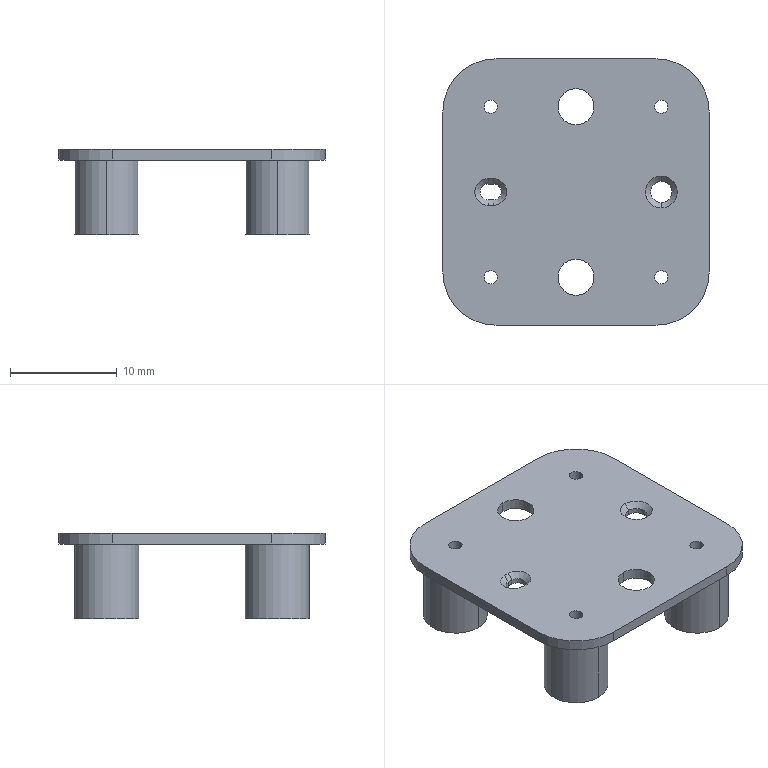NC program | NX | posted with a generic post | part box 25 x 25 x 8 mm
Whole program:
N10 G17 G21 G94 G90
(FLOOR_WALL_COPY , TOOL : D80)
N12 T19 M6
N14 G54
N16 G17 G0 G90 X-59.5 Y0. S6500 M3
N18 G43 Z30. H19
N20 Z3.
N22 G94 G1 Z0. F1500.
N24 X-54.5
N26 X54.5
N28 X59.5
N30 Z3.
N32 G0 Z30.
N34 M5
(DRILLING_COPY_1 , TOOL : D6A45)
N36 T01 M6
N38 G54
N40 G17 G0 G90 X-8. Y-8. S5000 M3
N42 G43 Z30. H1
N44 G94 G81 G98 Z-0.75 F350. R3.
N46 X0.
N48 X8.
N50 Y0.
N52 Y8.
N54 X0.
N56 X-8.
N58 G80
N60 G0 X-8. Y8. Z30.
N62 M5
(DRILLING_COPY_1_COPY_COPY , TOOL : 1.25ZT)
N64 T20 M6
N66 G54
N68 G17 G0 G90 X-8. Y-8. S2000 M3
N70 G43 Z30. H20
N72 G94 G83 G98 Z-9.376 F120. Q2. R3.
N74 Y8.
N76 X8.
N78 Y-8.
N80 G80
N82 G0 X8. Y-8. Z30.
N84 M5
(DRILLING_COPY_1_COPY_1_1_COPY_1 , TOOL : 3.4ZT)
N86 T03 M6
N88 G54
N90 G17 G0 G90 X0. Y-8. S2000 M3
N92 G43 Z30. H3
N94 G94 G83 G98 Z-3.521 F200. Q2. R3.
N96 Y8.
N98 G80
N100 G0 X0. Y8. Z30.
N102 M5
(ZLEVEL_PROFILE_COPY , TOOL : D1.0)
N104 T18 M6
N106 G54
N108 G17 G0 G90 X-7.518 Y-0.136 S9500 M3
N110 G43 Z30. H18
N112 Z0.5
N114 G94 G1 X-7.513 Y-0.131 F1000.
N116 Y0.121 Z0.486
N118 X-7.598 Y0.22 Z0.48
N120 X-7.722 Y0.24 Z0.473
N122 Y0.25
N124 X-8.278 Z0.443
N126 X-8.402 Y0.231 Z0.437
N128 X-8.487 Y0.131 Z0.43
N130 Y-0.12 Z0.417
N132 X-8.402 Y-0.219 Z0.41
N134 X-8.278 Y-0.239 Z0.403
N136 Y-0.25
N138 X-7.722 Z0.374
N140 X-7.598 Y-0.23 Z0.367
N142 X-7.513 Y-0.131 Z0.36
N144 Y0.121 Z0.347
N146 X-7.598 Y0.22 Z0.34
N148 X-7.722 Y0.24 Z0.334
N150 Y0.25 Z0.333
N152 X-8.278 Z0.304
N154 X-8.402 Y0.231 Z0.297
N156 X-8.487 Y0.131 Z0.29
N158 Y-0.12 Z0.277
N160 X-8.402 Y-0.219 Z0.27
N162 X-8.278 Y-0.239 Z0.264
N164 Y-0.25 Z0.263
N166 X-7.722 Z0.234
N168 X-7.598 Y-0.23 Z0.228
N170 X-7.513 Y-0.131 Z0.221
N172 Y0.121 Z0.207
N174 X-7.598 Y0.22 Z0.201
N176 X-7.722 Y0.24 Z0.194
N178 Y0.25
N180 X-8.278 Z0.164
N182 X-8.402 Y0.231 Z0.158
N184 X-8.487 Y0.131 Z0.151
N186 Y-0.12 Z0.138
N188 X-8.402 Y-0.219 Z0.131
N190 X-8.278 Y-0.239 Z0.124
N192 Y-0.25
N194 X-7.722 Z0.095
N196 X-7.598 Y-0.23 Z0.088
N198 X-7.513 Y-0.131 Z0.081
N200 Y0.121 Z0.068
N202 X-7.598 Y0.22 Z0.061
N204 X-7.722 Y0.24 Z0.055
N206 Y0.25 Z0.054
N208 X-8.278 Z0.025
N210 X-8.402 Y0.231 Z0.018
N212 X-8.487 Y0.131 Z0.011
N214 Y-0.12 Z-0.002
N216 X-8.402 Y-0.219 Z-0.009
N218 X-8.278 Y-0.239 Z-0.015
N220 Y-0.25 Z-0.016
N222 X-7.722 Z-0.045
N224 X-7.598 Y-0.23 Z-0.051
N226 X-7.513 Y-0.131 Z-0.058
N228 Y0.121 Z-0.071
N230 X-7.598 Y0.22 Z-0.078
N232 X-7.722 Y0.24 Z-0.085
N234 Y0.25
N236 X-8. Z-0.1
N238 X-8.278
N240 G3 X-8.278 Y-0.239 R0.247
N242 G1 Y-0.25
N244 X-7.722
N246 G3 X-7.722 Y0.24 R0.248
N248 G1 Y0.25
N250 X-8.
N252 X-8.119 Z-0.106
N254 X-8.238 Y0.245 Z-0.113
N256 X-8.385 Y0.195 Z-0.121
N258 X-8.437 Y0.146 Z-0.125
N260 X-8.479 Y0.059 Z-0.13
N262 X-8.489 Y0.015 Z-0.132
N264 X-8.488 Y-0.016 Z-0.134
N266 X-8.475 Y-0.078 Z-0.138
N268 X-8.435 Y-0.148 Z-0.142
N270 X-8.41 Y-0.179 Z-0.144
N272 X-8.378 Y-0.199 Z-0.146
N274 X-8.305 Y-0.231 Z-0.15
N276 X-8.261 Y-0.241 Z-0.153
N278 X-8.08 Y-0.25 Z-0.163
N280 X-7.842 Z-0.175
N282 X-7.663 Y-0.225 Z-0.185
N284 X-7.62 Y-0.198 Z-0.188
N286 X-7.54 Y-0.112 Z-0.194
N288 X-7.513 Y0. Z-0.2
N290 G3 X-7.722 Y0.24 R0.248
N292 G1 Y0.25
N294 X-8.
N296 X-8.119 Z-0.206
N298 X-8.238 Y0.245 Z-0.213
N300 X-8.385 Y0.195 Z-0.221
N302 X-8.437 Y0.146 Z-0.225
N304 X-8.479 Y0.059 Z-0.23
N306 X-8.489 Y0.015 Z-0.232
N308 X-8.488 Y-0.016 Z-0.234
N310 X-8.475 Y-0.078 Z-0.238
N312 X-8.435 Y-0.148 Z-0.242
N314 X-8.41 Y-0.179 Z-0.244
N316 X-8.378 Y-0.199 Z-0.246
N318 X-8.305 Y-0.231 Z-0.25
N320 X-8.261 Y-0.241 Z-0.253
N322 X-8.08 Y-0.25 Z-0.263
N324 X-7.842 Z-0.275
N326 X-7.663 Y-0.225 Z-0.285
N328 X-7.62 Y-0.198 Z-0.288
N330 X-7.54 Y-0.112 Z-0.294
N332 X-7.513 Y0. Z-0.3
N334 G3 X-7.722 Y0.24 R0.248
N336 G1 Y0.25
N338 X-8.
N340 X-8.119 Z-0.306
N342 X-8.238 Y0.245 Z-0.313
N344 X-8.385 Y0.195 Z-0.321
N346 X-8.437 Y0.146 Z-0.325
N348 X-8.479 Y0.059 Z-0.33
N350 X-8.489 Y0.015 Z-0.332
N352 X-8.488 Y-0.016 Z-0.334
N354 X-8.475 Y-0.078 Z-0.338
N356 X-8.435 Y-0.148 Z-0.342
N358 X-8.41 Y-0.179 Z-0.344
N360 X-8.378 Y-0.199 Z-0.346
N362 X-8.305 Y-0.231 Z-0.35
N364 X-8.261 Y-0.24 Z-0.353
N366 X-8.08 Y-0.25 Z-0.363
N368 X-7.842 Z-0.375
N370 X-7.663 Y-0.225 Z-0.385
N372 X-7.62 Y-0.198 Z-0.388
N374 X-7.54 Y-0.112 Z-0.394
N376 X-7.513 Y0. Z-0.4
N378 G3 X-7.722 Y0.24 R0.248
N380 G1 Y0.25
N382 X-8.
N384 X-8.119 Z-0.406
N386 X-8.238 Y0.245 Z-0.413
N388 X-8.385 Y0.195 Z-0.421
N390 X-8.437 Y0.146 Z-0.425
N392 X-8.479 Y0.059 Z-0.43
N394 X-8.488 Y0.016 Z-0.432
N396 X-8.49 Y-0.016 Z-0.434
N398 X-8.475 Y-0.078 Z-0.438
N400 X-8.434 Y-0.151 Z-0.442
N402 X-8.407 Y-0.18 Z-0.444
N404 X-8.376 Y-0.201 Z-0.446
N406 X-8.305 Y-0.231 Z-0.45
N408 X-8.26 Y-0.24 Z-0.453
N410 X-8.08 Y-0.25 Z-0.463
N412 X-7.842 Z-0.475
N414 X-7.666 Y-0.224 Z-0.484
N416 X-7.62 Y-0.198 Z-0.488
N418 X-7.54 Y-0.109 Z-0.494
N420 X-7.5 Y0. Z-0.5
N422 G3 X-7.75 Y0.25 R0.25
N424 G1 X-8.
N426 X-8.12 Z-0.506
N428 X-8.241 Y0.243 Z-0.513
N430 X-8.388 Y0.192 Z-0.521
N432 X-8.44 Y0.142 Z-0.525
N434 X-8.489 Y0.016 Z-0.532
N436 X-8.477 Y-0.075 Z-0.538
N438 X-8.418 Y-0.172 Z-0.544
N440 X-8.317 Y-0.228 Z-0.55
N442 X-8.275 Y-0.236 Z-0.552
N444 X-8.08 Y-0.25 Z-0.563
N446 X-7.839 Z-0.575
N448 X-7.662 Y-0.224 Z-0.584
N450 X-7.615 Y-0.195 Z-0.588
N452 X-7.538 Y-0.108 Z-0.594
N454 X-7.5 Y0. Z-0.6
N456 G3 X-7.75 Y0.25 R0.25
N458 G1 X-8.
N460 X-8.12 Z-0.606
N462 X-8.241 Y0.243 Z-0.613
N464 X-8.388 Y0.192 Z-0.621
N466 X-8.44 Y0.142 Z-0.625
N468 X-8.489 Y0.016 Z-0.632
N470 X-8.477 Y-0.075 Z-0.638
N472 X-8.418 Y-0.172 Z-0.644
N474 X-8.317 Y-0.228 Z-0.65
N476 X-8.275 Y-0.238 Z-0.652
N478 X-8.08 Y-0.25 Z-0.663
N480 X-7.839 Z-0.675
N482 X-7.662 Y-0.224 Z-0.684
N484 X-7.615 Y-0.195 Z-0.688
N486 X-7.538 Y-0.108 Z-0.694
N488 X-7.5 Y0. Z-0.7
N490 G3 X-7.75 Y0.25 R0.25
N492 G1 X-8.
N494 X-8.12 Z-0.706
N496 X-8.241 Y0.243 Z-0.713
N498 X-8.388 Y0.192 Z-0.721
N500 X-8.44 Y0.142 Z-0.725
N502 X-8.489 Y0.016 Z-0.732
N504 X-8.477 Y-0.075 Z-0.738
N506 X-8.418 Y-0.172 Z-0.744
N508 X-8.317 Y-0.228 Z-0.75
N510 X-8.274 Y-0.238 Z-0.752
N512 X-8.08 Y-0.25 Z-0.763
N514 X-7.839 Z-0.775
N516 X-7.662 Y-0.224 Z-0.784
N518 X-7.615 Y-0.195 Z-0.788
N520 X-7.538 Y-0.108 Z-0.794
N522 X-7.5 Y0. Z-0.8
N524 G3 X-7.75 Y0.25 R0.25
N526 G1 X-8.
N528 X-8.12 Z-0.806
N530 X-8.241 Y0.243 Z-0.813
N532 X-8.389 Y0.193 Z-0.821
N534 X-8.44 Y0.142 Z-0.825
N536 X-8.489 Y0.013 Z-0.832
N538 X-8.477 Y-0.075 Z-0.838
N540 X-8.417 Y-0.172 Z-0.844
N542 X-8.317 Y-0.228 Z-0.85
N544 X-8.274 Y-0.238 Z-0.852
N546 X-8.08 Y-0.25 Z-0.863
N548 X-7.839 Z-0.875
N550 X-7.662 Y-0.224 Z-0.884
N552 X-7.615 Y-0.195 Z-0.888
N554 X-7.538 Y-0.108 Z-0.894
N556 X-7.5 Y0. Z-0.9
N558 G3 X-7.75 Y0.25 R0.25
N560 G1 X-8.
N562 X-8.12 Z-0.906
N564 X-8.241 Y0.243 Z-0.913
N566 X-8.389 Y0.193 Z-0.921
N568 X-8.44 Y0.142 Z-0.925
N570 X-8.489 Y0.013 Z-0.932
N572 X-8.477 Y-0.075 Z-0.938
N574 X-8.44 Y-0.143 Z-0.942
N576 X-8.419 Y-0.173 Z-0.944
N578 X-8.387 Y-0.193 Z-0.946
N580 X-8.317 Y-0.228 Z-0.95
N582 X-8.269 Y-0.238 Z-0.953
N584 X-8.08 Y-0.25 Z-0.963
N586 X-7.839 Z-0.975
N588 X-7.662 Y-0.224 Z-0.984
N590 X-7.615 Y-0.195 Z-0.988
N592 X-7.538 Y-0.108 Z-0.994
N594 X-7.5 Y0. Z-1.
N596 G3 X-7.75 Y0.25 R0.25
N598 G1 X-8.25
N600 G3 X-8.5 Y0. R0.25
N602 X-8.25 Y-0.25 R0.25
N604 G1 X-7.75
N606 G3 X-7.5 Y0. R0.25
N608 G1 Z-0.5
N610 G0 Z30.
N612 X7.651 Y0.313
N614 Z0.5
N616 G1 X7.51 Y0.157 Z0.489
N618 X7.521 Y-0.192 Z0.471
N620 X7.825 Y-0.492 Z0.448
N622 X8. Y-0.495 Z0.439
N624 X8.174 Y-0.492 Z0.43
N626 X8.485 Y-0.177 Z0.407
N628 Y0.012 Z0.397
N630 X8.479 Y0.187 Z0.388
N632 X8.144 Y0.497 Z0.364
N634 X7.97 Y0.489 Z0.355
N636 X7.796 Y0.475 Z0.346
N638 X7.51 Y0.157 Z0.323
N640 X7.521 Y-0.192 Z0.305
N642 X7.825 Y-0.492 Z0.282
N644 X8. Y-0.495 Z0.273
N646 X8.174 Y-0.492 Z0.264
N648 X8.485 Y-0.177 Z0.241
N650 Y0.012 Z0.231
N652 X8.479 Y0.187 Z0.222
N654 X8.144 Y0.497 Z0.198
N656 X7.97 Y0.489 Z0.189
N658 X7.796 Y0.475 Z0.18
N660 X7.51 Y0.157 Z0.157
N662 X7.521 Y-0.192 Z0.139
N664 X7.825 Y-0.492 Z0.117
N666 X8. Y-0.495 Z0.107
N668 X8.174 Y-0.492 Z0.098
N670 X8.485 Y-0.177 Z0.075
N672 Y0.012 Z0.065
N674 X8.479 Y0.187 Z0.056
N676 X8.144 Y0.497 Z0.032
N678 X7.97 Y0.489 Z0.023
N680 X7.796 Y0.475 Z0.014
N682 X7.51 Y0.157 Z-0.009
N684 X7.521 Y-0.192 Z-0.027
N686 X7.825 Y-0.492 Z-0.049
N688 X8. Y-0.495 Z-0.059
N690 X8.174 Y-0.492 Z-0.068
N692 X8.485 Y-0.177 Z-0.091
N694 Y-0.003 Z-0.1
N696 Y0.012
N698 G3 X7.97 Y0.489 R0.492
N700 X8. Y-0.495 R0.493
N702 X8.485 Y-0.003 R0.492
N704 G1 X8.461 Y0.154 Z-0.107
N706 X8.434 Y0.22 Z-0.11
N708 X8.36 Y0.328 Z-0.116
N710 X8.284 Y0.39 Z-0.12
N712 X8.162 Y0.461 Z-0.126
N714 X8.075 Y0.477 Z-0.13
N716 X7.931 Y0.479 Z-0.136
N718 X7.851 Y0.461 Z-0.14
N720 X7.722 Y0.395 Z-0.146
N722 X7.652 Y0.348 Z-0.15
N724 X7.588 Y0.252 Z-0.155
N726 X7.538 Y0.148 Z-0.16
N728 X7.513 Y0.027 Z-0.165
N730 X7.525 Y-0.078 Z-0.17
N732 X7.562 Y-0.213 Z-0.176
N734 X7.612 Y-0.286 Z-0.18
N736 X7.709 Y-0.385 Z-0.186
N738 X7.783 Y-0.433 Z-0.19
N740 X7.89 Y-0.471 Z-0.195
N742 X8. Y-0.495 Z-0.2
N744 G3 X8.485 Y-0.003 R0.492
N746 G1 X8.461 Y0.154 Z-0.207
N748 X8.434 Y0.22 Z-0.21
N750 X8.36 Y0.327 Z-0.216
N752 X8.284 Y0.39 Z-0.22
N754 X8.162 Y0.461 Z-0.226
N756 X8.075 Y0.477 Z-0.23
N758 X7.931 Y0.479 Z-0.236
N760 X7.851 Y0.461 Z-0.24
N762 X7.723 Y0.395 Z-0.246
N764 X7.652 Y0.348 Z-0.25
N766 X7.588 Y0.252 Z-0.255
N768 X7.538 Y0.148 Z-0.26
N770 X7.513 Y0.027 Z-0.265
N772 X7.525 Y-0.078 Z-0.27
N774 X7.562 Y-0.213 Z-0.276
N776 X7.612 Y-0.286 Z-0.28
N778 X7.709 Y-0.385 Z-0.286
N780 X7.783 Y-0.433 Z-0.29
N782 X7.89 Y-0.47 Z-0.295
N784 X8. Y-0.495 Z-0.3
N786 G3 X8.485 Y-0.003 R0.492
N788 G1 X8.461 Y0.154 Z-0.307
N790 X8.434 Y0.22 Z-0.31
N792 X8.36 Y0.327 Z-0.316
N794 X8.284 Y0.39 Z-0.32
N796 X8.162 Y0.461 Z-0.326
N798 X8.075 Y0.477 Z-0.33
N800 X7.932 Y0.479 Z-0.336
N802 X7.851 Y0.461 Z-0.34
N804 X7.723 Y0.395 Z-0.346
N806 X7.652 Y0.348 Z-0.35
N808 X7.588 Y0.252 Z-0.355
N810 X7.538 Y0.148 Z-0.36
N812 X7.513 Y0.027 Z-0.365
N814 X7.525 Y-0.078 Z-0.37
N816 X7.562 Y-0.213 Z-0.376
N818 X7.612 Y-0.286 Z-0.38
N820 X7.709 Y-0.385 Z-0.386
N822 X7.783 Y-0.433 Z-0.39
N824 X7.89 Y-0.47 Z-0.395
N826 X8. Y-0.495 Z-0.4
N828 G3 X8.485 Y-0.003 R0.492
N830 G1 X8.461 Y0.151 Z-0.407
N832 X8.433 Y0.219 Z-0.41
N834 X8.358 Y0.328 Z-0.416
N836 X8.284 Y0.39 Z-0.42
N838 X8.162 Y0.461 Z-0.426
N840 X8.075 Y0.478 Z-0.43
N842 X7.932 Y0.477 Z-0.436
N844 X7.85 Y0.462 Z-0.44
N846 X7.727 Y0.398 Z-0.446
N848 X7.652 Y0.347 Z-0.45
N850 X7.588 Y0.251 Z-0.455
N852 X7.538 Y0.149 Z-0.46
N854 X7.515 Y0.028 Z-0.465
N856 X7.524 Y-0.078 Z-0.47
N858 X7.561 Y-0.211 Z-0.476
N860 X7.611 Y-0.287 Z-0.48
N862 X7.706 Y-0.383 Z-0.486
N864 X7.782 Y-0.433 Z-0.49
N866 X7.89 Y-0.47 Z-0.495
N868 X8. Y-0.5 Z-0.5
N870 X8.015
N872 G3 X8.5 Y-0.003 R0.5
N874 G1 X8.466 Y0.127 Z-0.506
N876 X8.434 Y0.218 Z-0.51
N878 X8.364 Y0.323 Z-0.516
N880 X8.286 Y0.389 Z-0.52
N882 X8.169 Y0.459 Z-0.526
N884 X8.078 Y0.477 Z-0.53
N886 X7.935 Y0.479 Z-0.536
N888 X7.853 Y0.462 Z-0.54
N890 X7.733 Y0.401 Z-0.546
N892 X7.655 Y0.349 Z-0.55
N894 X7.525 Y0.157 Z-0.56
N896 X7.504 Y0.063 Z-0.564
N898 X7.522 Y-0.073 Z-0.57
N900 X7.561 Y-0.211 Z-0.576
N902 X7.609 Y-0.281 Z-0.58
N904 X7.708 Y-0.385 Z-0.586
N906 X7.777 Y-0.431 Z-0.59
N908 X7.886 Y-0.469 Z-0.595
N910 X7.997 Y-0.5 Z-0.6
N912 X8.015
N914 G3 X8.5 Y-0.003 R0.5
N916 G1 X8.466 Y0.127 Z-0.606
N918 X8.434 Y0.218 Z-0.61
N920 X8.364 Y0.323 Z-0.616
N922 X8.286 Y0.389 Z-0.62
N924 X8.169 Y0.459 Z-0.626
N926 X8.078 Y0.477 Z-0.63
N928 X7.935 Y0.479 Z-0.636
N930 X7.853 Y0.462 Z-0.64
N932 X7.733 Y0.401 Z-0.646
N934 X7.655 Y0.349 Z-0.65
N936 X7.525 Y0.157 Z-0.66
N938 X7.504 Y0.063 Z-0.664
N940 X7.522 Y-0.073 Z-0.67
N942 X7.561 Y-0.211 Z-0.676
N944 X7.609 Y-0.281 Z-0.68
N946 X7.708 Y-0.385 Z-0.686
N948 X7.777 Y-0.431 Z-0.69
N950 X7.886 Y-0.469 Z-0.695
N952 X7.997 Y-0.5 Z-0.7
N954 X8.015
N956 G3 X8.5 Y-0.003 R0.5
N958 G1 X8.466 Y0.126 Z-0.706
N960 X8.434 Y0.218 Z-0.71
N962 X8.364 Y0.323 Z-0.716
N964 X8.286 Y0.389 Z-0.72
N966 X8.168 Y0.458 Z-0.726
N968 X8.078 Y0.477 Z-0.73
N970 X7.936 Y0.479 Z-0.736
N972 X7.853 Y0.462 Z-0.74
N974 X7.733 Y0.401 Z-0.746
N976 X7.655 Y0.349 Z-0.75
N978 X7.525 Y0.157 Z-0.76
N980 X7.504 Y0.063 Z-0.764
N982 X7.522 Y-0.073 Z-0.77
N984 X7.561 Y-0.211 Z-0.776
N986 X7.609 Y-0.281 Z-0.78
N988 X7.708 Y-0.385 Z-0.786
N990 X7.777 Y-0.431 Z-0.79
N992 X7.886 Y-0.468 Z-0.795
N994 X7.997 Y-0.5 Z-0.8
N996 X8.015
N998 G3 X8.5 Y-0.003 R0.5
N1000 G1 X8.466 Y0.126 Z-0.806
N1002 X8.434 Y0.218 Z-0.81
N1004 X8.364 Y0.323 Z-0.816
N1006 X8.286 Y0.389 Z-0.82
N1008 X8.168 Y0.458 Z-0.826
N1010 X8.078 Y0.477 Z-0.83
N1012 X7.936 Y0.479 Z-0.836
N1014 X7.853 Y0.462 Z-0.84
N1016 X7.733 Y0.401 Z-0.846
N1018 X7.655 Y0.349 Z-0.85
N1020 X7.525 Y0.157 Z-0.86
N1022 X7.504 Y0.063 Z-0.864
N1024 X7.522 Y-0.073 Z-0.87
N1026 X7.561 Y-0.211 Z-0.876
N1028 X7.609 Y-0.281 Z-0.88
N1030 X7.708 Y-0.385 Z-0.886
N1032 X7.777 Y-0.431 Z-0.89
N1034 X7.886 Y-0.468 Z-0.895
N1036 X7.997 Y-0.5 Z-0.9
N1038 X8.015
N1040 G3 X8.5 Y-0.003 R0.5
N1042 G1 X8.466 Y0.126 Z-0.906
N1044 X8.434 Y0.218 Z-0.91
N1046 X8.364 Y0.323 Z-0.916
N1048 X8.286 Y0.389 Z-0.92
N1050 X8.168 Y0.458 Z-0.926
N1052 X8.078 Y0.477 Z-0.93
N1054 X7.936 Y0.479 Z-0.936
N1056 X7.853 Y0.462 Z-0.94
N1058 X7.733 Y0.401 Z-0.946
N1060 X7.655 Y0.349 Z-0.95
N1062 X7.525 Y0.157 Z-0.96
N1064 X7.504 Y0.063 Z-0.964
N1066 X7.522 Y-0.073 Z-0.97
N1068 X7.561 Y-0.211 Z-0.976
N1070 X7.609 Y-0.281 Z-0.98
N1072 X7.708 Y-0.385 Z-0.986
N1074 X7.777 Y-0.431 Z-0.99
N1076 X7.886 Y-0.468 Z-0.995
N1078 X7.997 Y-0.5 Z-1.
N1080 X8.015
N1082 G3 X7.997 Y-0.5 R-0.5
N1084 G1 Z-0.5
N1086 G0 Z30.
N1088 M5
(ZLEVEL_PROFILE , TOOL : D10)
N1090 T15 M6
N1092 G54
N1094 G17 G0 G90 X15.543 Y-13.61 S9500 M3
N1096 G43 Z30. H15
N1098 Z1.5
N1100 G94 G1 X15.35 Y-13.903 Z1.482 F1000.
N1102 X13.903 Y-15.35 Z1.374
N1104 X12.194 Y-16.477 Z1.267
N1106 X10.293 Y-17.237 Z1.16
N1108 X8.279 Y-17.6 Z1.053
N1110 X-8.279 Z0.185
N1112 X-10.293 Y-17.237 Z0.078
N1114 X-12.194 Y-16.477 Z-0.03
N1116 X-13.903 Y-15.35 Z-0.137
N1118 X-15.35 Y-13.903 Z-0.244
N1120 X-16.477 Y-12.194 Z-0.352
N1122 X-17.237 Y-10.293 Z-0.459
N1124 X-17.6 Y-8.279 Z-0.566
N1126 Y0. Z-1.
N1128 Y7.5 F3200.
N1130 G2 X-7.5 Y17.6 R10.1
N1132 G1 X7.5
N1134 G2 X17.6 Y7.5 R10.1
N1136 G1 Y-7.5
N1138 G2 X7.5 Y-17.6 R10.1
N1140 G1 X-7.5
N1142 G2 X-17.6 Y-7.5 R10.1
N1144 G1 Y0.
N1146 Y6.968 Z-1.122
N1148 Y7.355 Z-1.128
N1150 X-17.597 Y7.742 Z-1.135
N1152 X-17.58 Y8.129 Z-1.142
N1154 X-17.549 Y8.514 Z-1.149
N1156 X-17.503 Y8.899 Z-1.155
N1158 X-17.442 Y9.281 Z-1.162
N1160 X-17.366 Y9.661 Z-1.169
N1162 X-17.276 Y10.037 Z-1.176
N1164 X-17.172 Y10.41 Z-1.182
N1166 X-17.053 Y10.778 Z-1.189
N1168 X-16.921 Y11.142 Z-1.196
N1170 X-16.774 Y11.5 Z-1.203
N1172 X-16.614 Y11.853 Z-1.209
N1174 X-16.441 Y12.199 Z-1.216
N1176 X-16.254 Y12.538 Z-1.223
N1178 X-16.055 Y12.869 Z-1.23
N1180 X-15.842 Y13.193 Z-1.236
N1182 X-15.618 Y13.509 Z-1.243
N1184 X-15.382 Y13.815 Z-1.25
N1186 X-15.134 Y14.113 Z-1.257
N1188 X-14.875 Y14.4 Z-1.264
N1190 X-14.605 Y14.678 Z-1.27
N1192 X-14.325 Y14.945 Z-1.277
N1194 X-14.035 Y15.201 Z-1.284
N1196 X-13.735 Y15.446 Z-1.291
N1198 X-13.426 Y15.679 Z-1.297
N1200 X-13.108 Y15.9 Z-1.304
N1202 X-12.782 Y16.109 Z-1.311
N1204 X-12.449 Y16.305 Z-1.318
N1206 X-12.108 Y16.488 Z-1.324
N1208 X-11.76 Y16.658 Z-1.331
N1210 X-11.406 Y16.814 Z-1.338
N1212 X-11.046 Y16.957 Z-1.345
N1214 X-10.681 Y17.086 Z-1.351
N1216 X-10.311 Y17.201 Z-1.358
N1218 X-9.938 Y17.301 Z-1.365
N1220 X-9.56 Y17.388 Z-1.372
N1222 X-9.18 Y17.459 Z-1.378
N1224 X-8.797 Y17.516 Z-1.385
N1226 X-8.412 Y17.559 Z-1.392
N1228 X-8.026 Y17.586 Z-1.399
N1230 X-7.639 Y17.599 Z-1.405
N1232 X-7.252 Y17.6 Z-1.412
N1234 X-6.478 Z-1.426
N1236 X7.07 Z-1.662
N1238 X7.457 Z-1.669
N1240 X7.844 Y17.594 Z-1.676
N1242 X8.231 Y17.574 Z-1.682
N1244 X8.616 Y17.538 Z-1.689
N1246 X9. Y17.488 Z-1.696
N1248 X9.382 Y17.423 Z-1.703
N1250 X9.761 Y17.344 Z-1.709
N1252 X10.136 Y17.25 Z-1.716
N1254 X10.508 Y17.142 Z-1.723
N1256 X10.875 Y17.019 Z-1.73
N1258 X11.237 Y16.883 Z-1.736
N1260 X11.594 Y16.733 Z-1.743
N1262 X11.945 Y16.569 Z-1.75
N1264 X12.289 Y16.392 Z-1.757
N1266 X12.626 Y16.202 Z-1.764
N1268 X12.956 Y16. Z-1.77
N1270 X13.278 Y15.784 Z-1.777
N1272 X13.591 Y15.557 Z-1.784
N1274 X13.895 Y15.318 Z-1.791
N1276 X14.19 Y15.067 Z-1.797
N1278 X14.475 Y14.805 Z-1.804
N1280 X14.75 Y14.532 Z-1.811
N1282 X15.014 Y14.249 Z-1.818
N1284 X15.267 Y13.956 Z-1.824
N1286 X15.509 Y13.654 Z-1.831
N1288 X15.739 Y13.343 Z-1.838
N1290 X15.956 Y13.023 Z-1.845
N1292 X16.162 Y12.695 Z-1.851
N1294 X16.354 Y12.359 Z-1.858
N1296 X16.534 Y12.016 Z-1.865
N1298 X16.7 Y11.667 Z-1.872
N1300 X16.853 Y11.311 Z-1.878
N1302 X16.993 Y10.95 Z-1.885
N1304 X17.118 Y10.584 Z-1.892
N1306 X17.229 Y10.213 Z-1.899
N1308 X17.326 Y9.838 Z-1.905
N1310 X17.408 Y9.46 Z-1.912
N1312 X17.476 Y9.079 Z-1.919
N1314 X17.529 Y8.695 Z-1.926
N1316 X17.567 Y8.31 Z-1.932
N1318 X17.591 Y7.924 Z-1.939
N1320 X17.6 Y7.537 Z-1.946
N1322 Y7.15 Z-1.953
N1324 Y4.44 Z-2.
N1326 Y-7.5
N1328 G2 X7.5 Y-17.6 R10.1
N1330 G1 X-7.5
N1332 G2 X-17.6 Y-7.5 R10.1
N1334 G1 Y0.
N1336 Y6.968 Z-2.122
N1338 Y7.355 Z-2.128
N1340 X-17.597 Y7.742 Z-2.135
N1342 X-17.58 Y8.129 Z-2.142
N1344 X-17.549 Y8.514 Z-2.149
N1346 X-17.503 Y8.899 Z-2.155
N1348 X-17.442 Y9.281 Z-2.162
N1350 X-17.366 Y9.661 Z-2.169
N1352 X-17.276 Y10.037 Z-2.176
N1354 X-17.172 Y10.41 Z-2.182
N1356 X-17.053 Y10.778 Z-2.189
N1358 X-16.921 Y11.142 Z-2.196
N1360 X-16.774 Y11.5 Z-2.203
N1362 X-16.614 Y11.853 Z-2.209
N1364 X-16.441 Y12.199 Z-2.216
N1366 X-16.254 Y12.538 Z-2.223
N1368 X-16.055 Y12.869 Z-2.23
N1370 X-15.842 Y13.193 Z-2.236
N1372 X-15.618 Y13.509 Z-2.243
N1374 X-15.382 Y13.815 Z-2.25
N1376 X-15.134 Y14.113 Z-2.257
N1378 X-14.875 Y14.4 Z-2.264
N1380 X-14.605 Y14.678 Z-2.27
N1382 X-14.325 Y14.945 Z-2.277
N1384 X-14.035 Y15.201 Z-2.284
N1386 X-13.735 Y15.446 Z-2.291
N1388 X-13.426 Y15.679 Z-2.297
N1390 X-13.108 Y15.9 Z-2.304
N1392 X-12.782 Y16.109 Z-2.311
N1394 X-12.449 Y16.305 Z-2.318
N1396 X-12.108 Y16.488 Z-2.324
N1398 X-11.76 Y16.658 Z-2.331
N1400 X-11.406 Y16.814 Z-2.338
N1402 X-11.046 Y16.957 Z-2.345
N1404 X-10.681 Y17.086 Z-2.351
N1406 X-10.311 Y17.201 Z-2.358
N1408 X-9.938 Y17.301 Z-2.365
N1410 X-9.56 Y17.388 Z-2.372
N1412 X-9.18 Y17.459 Z-2.378
N1414 X-8.797 Y17.516 Z-2.385
N1416 X-8.412 Y17.559 Z-2.392
N1418 X-8.026 Y17.586 Z-2.399
N1420 X-7.639 Y17.599 Z-2.405
N1422 X-7.252 Y17.6 Z-2.412
N1424 X-6.478 Z-2.426
N1426 X7.07 Z-2.662
N1428 X7.457 Z-2.669
N1430 X7.844 Y17.594 Z-2.676
N1432 X8.231 Y17.574 Z-2.682
N1434 X8.616 Y17.538 Z-2.689
N1436 X9. Y17.488 Z-2.696
N1438 X9.382 Y17.423 Z-2.703
N1440 X9.761 Y17.344 Z-2.709
N1442 X10.136 Y17.25 Z-2.716
N1444 X10.508 Y17.142 Z-2.723
N1446 X10.875 Y17.019 Z-2.73
N1448 X11.237 Y16.883 Z-2.736
N1450 X11.594 Y16.733 Z-2.743
N1452 X11.945 Y16.569 Z-2.75
N1454 X12.289 Y16.392 Z-2.757
N1456 X12.626 Y16.202 Z-2.764
N1458 X12.956 Y16. Z-2.77
N1460 X13.278 Y15.784 Z-2.777
N1462 X13.591 Y15.557 Z-2.784
N1464 X13.895 Y15.318 Z-2.791
N1466 X14.19 Y15.067 Z-2.797
N1468 X14.475 Y14.805 Z-2.804
N1470 X14.75 Y14.532 Z-2.811
N1472 X15.014 Y14.249 Z-2.818
N1474 X15.267 Y13.956 Z-2.824
N1476 X15.509 Y13.654 Z-2.831
N1478 X15.739 Y13.343 Z-2.838
N1480 X15.956 Y13.023 Z-2.845
N1482 X16.162 Y12.695 Z-2.851
N1484 X16.354 Y12.359 Z-2.858
N1486 X16.534 Y12.016 Z-2.865
N1488 X16.7 Y11.667 Z-2.872
N1490 X16.853 Y11.311 Z-2.878
N1492 X16.993 Y10.95 Z-2.885
N1494 X17.118 Y10.584 Z-2.892
N1496 X17.229 Y10.213 Z-2.899
N1498 X17.326 Y9.838 Z-2.905
N1500 X17.408 Y9.46 Z-2.912
N1502 X17.476 Y9.079 Z-2.919
N1504 X17.529 Y8.695 Z-2.926
N1506 X17.567 Y8.31 Z-2.932
N1508 X17.591 Y7.924 Z-2.939
N1510 X17.6 Y7.537 Z-2.946
N1512 Y7.15 Z-2.953
N1514 Y4.44 Z-3.
N1516 Y-7.5
N1518 G2 X7.5 Y-17.6 R10.1
N1520 G1 X-7.5
N1522 G2 X-17.6 Y-7.5 R10.1
N1524 G1 Y0.
N1526 Y6.968 Z-3.122
N1528 Y7.355 Z-3.128
N1530 X-17.597 Y7.742 Z-3.135
N1532 X-17.58 Y8.129 Z-3.142
N1534 X-17.549 Y8.514 Z-3.149
N1536 X-17.503 Y8.899 Z-3.155
N1538 X-17.442 Y9.281 Z-3.162
N1540 X-17.366 Y9.661 Z-3.169
N1542 X-17.276 Y10.037 Z-3.176
N1544 X-17.172 Y10.41 Z-3.182
N1546 X-17.053 Y10.778 Z-3.189
N1548 X-16.921 Y11.142 Z-3.196
N1550 X-16.774 Y11.5 Z-3.203
N1552 X-16.614 Y11.853 Z-3.209
N1554 X-16.441 Y12.199 Z-3.216
N1556 X-16.254 Y12.538 Z-3.223
N1558 X-16.055 Y12.869 Z-3.23
N1560 X-15.842 Y13.193 Z-3.236
N1562 X-15.618 Y13.509 Z-3.243
N1564 X-15.382 Y13.815 Z-3.25
N1566 X-15.134 Y14.113 Z-3.257
N1568 X-14.875 Y14.4 Z-3.264
N1570 X-14.605 Y14.678 Z-3.27
N1572 X-14.325 Y14.945 Z-3.277
N1574 X-14.035 Y15.201 Z-3.284
N1576 X-13.735 Y15.446 Z-3.291
N1578 X-13.426 Y15.679 Z-3.297
N1580 X-13.108 Y15.9 Z-3.304
N1582 X-12.782 Y16.109 Z-3.311
N1584 X-12.449 Y16.305 Z-3.318
N1586 X-12.108 Y16.488 Z-3.324
N1588 X-11.76 Y16.658 Z-3.331
N1590 X-11.406 Y16.814 Z-3.338
N1592 X-11.046 Y16.957 Z-3.345
N1594 X-10.681 Y17.086 Z-3.351
N1596 X-10.311 Y17.201 Z-3.358
N1598 X-9.938 Y17.301 Z-3.365
N1600 X-9.56 Y17.388 Z-3.372
N1602 X-9.18 Y17.459 Z-3.378
N1604 X-8.797 Y17.516 Z-3.385
N1606 X-8.412 Y17.559 Z-3.392
N1608 X-8.026 Y17.586 Z-3.399
N1610 X-7.639 Y17.599 Z-3.405
N1612 X-7.252 Y17.6 Z-3.412
N1614 X-6.478 Z-3.426
N1616 X7.07 Z-3.662
N1618 X7.457 Z-3.669
N1620 X7.844 Y17.594 Z-3.676
N1622 X8.231 Y17.574 Z-3.682
N1624 X8.616 Y17.538 Z-3.689
N1626 X9. Y17.488 Z-3.696
N1628 X9.382 Y17.423 Z-3.703
N1630 X9.761 Y17.344 Z-3.709
N1632 X10.136 Y17.25 Z-3.716
N1634 X10.508 Y17.142 Z-3.723
N1636 X10.875 Y17.019 Z-3.73
N1638 X11.237 Y16.883 Z-3.736
N1640 X11.594 Y16.733 Z-3.743
N1642 X11.945 Y16.569 Z-3.75
N1644 X12.289 Y16.392 Z-3.757
N1646 X12.626 Y16.202 Z-3.764
N1648 X12.956 Y16. Z-3.77
N1650 X13.278 Y15.784 Z-3.777
N1652 X13.591 Y15.557 Z-3.784
N1654 X13.895 Y15.318 Z-3.791
N1656 X14.19 Y15.067 Z-3.797
N1658 X14.475 Y14.805 Z-3.804
N1660 X14.75 Y14.532 Z-3.811
N1662 X15.014 Y14.249 Z-3.818
N1664 X15.267 Y13.956 Z-3.824
N1666 X15.509 Y13.654 Z-3.831
N1668 X15.739 Y13.343 Z-3.838
N1670 X15.956 Y13.023 Z-3.845
N1672 X16.162 Y12.695 Z-3.851
N1674 X16.354 Y12.359 Z-3.858
N1676 X16.534 Y12.016 Z-3.865
N1678 X16.7 Y11.667 Z-3.872
N1680 X16.853 Y11.311 Z-3.878
N1682 X16.993 Y10.95 Z-3.885
N1684 X17.118 Y10.584 Z-3.892
N1686 X17.229 Y10.213 Z-3.899
N1688 X17.326 Y9.838 Z-3.905
N1690 X17.408 Y9.46 Z-3.912
N1692 X17.476 Y9.079 Z-3.919
N1694 X17.529 Y8.695 Z-3.926
N1696 X17.567 Y8.31 Z-3.932
N1698 X17.591 Y7.924 Z-3.939
N1700 X17.6 Y7.537 Z-3.946
N1702 Y7.15 Z-3.953
N1704 Y4.44 Z-4.
N1706 Y-7.5
N1708 G2 X7.5 Y-17.6 R10.1
N1710 G1 X-7.5
N1712 G2 X-17.6 Y-7.5 R10.1
N1714 G1 Y0.
N1716 Y6.968 Z-4.122
N1718 Y7.355 Z-4.128
N1720 X-17.597 Y7.742 Z-4.135
N1722 X-17.58 Y8.129 Z-4.142
N1724 X-17.549 Y8.514 Z-4.149
N1726 X-17.503 Y8.899 Z-4.155
N1728 X-17.442 Y9.281 Z-4.162
N1730 X-17.366 Y9.661 Z-4.169
N1732 X-17.276 Y10.037 Z-4.176
N1734 X-17.172 Y10.41 Z-4.182
N1736 X-17.053 Y10.778 Z-4.189
N1738 X-16.921 Y11.142 Z-4.196
N1740 X-16.774 Y11.5 Z-4.203
N1742 X-16.614 Y11.853 Z-4.209
N1744 X-16.441 Y12.199 Z-4.216
N1746 X-16.254 Y12.538 Z-4.223
N1748 X-16.055 Y12.869 Z-4.23
N1750 X-15.842 Y13.193 Z-4.236
N1752 X-15.618 Y13.509 Z-4.243
N1754 X-15.382 Y13.815 Z-4.25
N1756 X-15.134 Y14.113 Z-4.257
N1758 X-14.875 Y14.4 Z-4.264
N1760 X-14.605 Y14.678 Z-4.27
N1762 X-14.325 Y14.945 Z-4.277
N1764 X-14.035 Y15.201 Z-4.284
N1766 X-13.735 Y15.446 Z-4.291
N1768 X-13.426 Y15.679 Z-4.297
N1770 X-13.108 Y15.9 Z-4.304
N1772 X-12.782 Y16.109 Z-4.311
N1774 X-12.449 Y16.305 Z-4.318
N1776 X-12.108 Y16.488 Z-4.324
N1778 X-11.76 Y16.658 Z-4.331
N1780 X-11.406 Y16.814 Z-4.338
N1782 X-11.046 Y16.957 Z-4.345
N1784 X-10.681 Y17.086 Z-4.351
N1786 X-10.311 Y17.201 Z-4.358
N1788 X-9.938 Y17.301 Z-4.365
N1790 X-9.56 Y17.388 Z-4.372
N1792 X-9.18 Y17.459 Z-4.378
N1794 X-8.797 Y17.516 Z-4.385
N1796 X-8.412 Y17.559 Z-4.392
N1798 X-8.026 Y17.586 Z-4.399
N1800 X-7.639 Y17.599 Z-4.405
N1802 X-7.252 Y17.6 Z-4.412
N1804 X-6.478 Z-4.426
N1806 X7.07 Z-4.662
N1808 X7.457 Z-4.669
N1810 X7.844 Y17.594 Z-4.676
N1812 X8.231 Y17.574 Z-4.682
N1814 X8.616 Y17.538 Z-4.689
N1816 X9. Y17.488 Z-4.696
N1818 X9.382 Y17.423 Z-4.703
N1820 X9.761 Y17.344 Z-4.709
N1822 X10.136 Y17.25 Z-4.716
N1824 X10.508 Y17.142 Z-4.723
N1826 X10.875 Y17.019 Z-4.73
N1828 X11.237 Y16.883 Z-4.736
N1830 X11.594 Y16.733 Z-4.743
N1832 X11.945 Y16.569 Z-4.75
N1834 X12.289 Y16.392 Z-4.757
N1836 X12.626 Y16.202 Z-4.764
N1838 X12.956 Y16. Z-4.77
N1840 X13.278 Y15.784 Z-4.777
N1842 X13.591 Y15.557 Z-4.784
N1844 X13.895 Y15.318 Z-4.791
N1846 X14.19 Y15.067 Z-4.797
N1848 X14.475 Y14.805 Z-4.804
N1850 X14.75 Y14.532 Z-4.811
N1852 X15.014 Y14.249 Z-4.818
N1854 X15.267 Y13.956 Z-4.824
N1856 X15.509 Y13.654 Z-4.831
N1858 X15.739 Y13.343 Z-4.838
N1860 X15.956 Y13.023 Z-4.845
N1862 X16.162 Y12.695 Z-4.851
N1864 X16.354 Y12.359 Z-4.858
N1866 X16.534 Y12.016 Z-4.865
N1868 X16.7 Y11.667 Z-4.872
N1870 X16.853 Y11.311 Z-4.878
N1872 X16.993 Y10.95 Z-4.885
N1874 X17.118 Y10.584 Z-4.892
N1876 X17.229 Y10.213 Z-4.899
N1878 X17.326 Y9.838 Z-4.905
N1880 X17.408 Y9.46 Z-4.912
N1882 X17.476 Y9.079 Z-4.919
N1884 X17.529 Y8.695 Z-4.926
N1886 X17.567 Y8.31 Z-4.932
N1888 X17.591 Y7.924 Z-4.939
N1890 X17.6 Y7.537 Z-4.946
N1892 Y7.15 Z-4.953
N1894 Y4.44 Z-5.
N1896 Y-7.5
N1898 G2 X7.5 Y-17.6 R10.1
N1900 G1 X-7.5
N1902 G2 X-17.6 Y-7.5 R10.1
N1904 G1 Y0.
N1906 Y6.968 Z-5.122
N1908 Y7.355 Z-5.128
N1910 X-17.597 Y7.742 Z-5.135
N1912 X-17.58 Y8.129 Z-5.142
N1914 X-17.549 Y8.514 Z-5.149
N1916 X-17.503 Y8.899 Z-5.155
N1918 X-17.442 Y9.281 Z-5.162
N1920 X-17.366 Y9.661 Z-5.169
N1922 X-17.276 Y10.037 Z-5.176
N1924 X-17.172 Y10.41 Z-5.182
N1926 X-17.053 Y10.778 Z-5.189
N1928 X-16.921 Y11.142 Z-5.196
N1930 X-16.774 Y11.5 Z-5.203
N1932 X-16.614 Y11.853 Z-5.209
N1934 X-16.441 Y12.199 Z-5.216
N1936 X-16.254 Y12.538 Z-5.223
N1938 X-16.055 Y12.869 Z-5.23
N1940 X-15.842 Y13.193 Z-5.236
N1942 X-15.618 Y13.509 Z-5.243
N1944 X-15.382 Y13.815 Z-5.25
N1946 X-15.134 Y14.113 Z-5.257
N1948 X-14.875 Y14.4 Z-5.264
N1950 X-14.605 Y14.678 Z-5.27
N1952 X-14.325 Y14.945 Z-5.277
N1954 X-14.035 Y15.201 Z-5.284
N1956 X-13.735 Y15.446 Z-5.291
N1958 X-13.426 Y15.679 Z-5.297
N1960 X-13.108 Y15.9 Z-5.304
N1962 X-12.782 Y16.109 Z-5.311
N1964 X-12.449 Y16.305 Z-5.318
N1966 X-12.108 Y16.488 Z-5.324
N1968 X-11.76 Y16.658 Z-5.331
N1970 X-11.406 Y16.814 Z-5.338
N1972 X-11.046 Y16.957 Z-5.345
N1974 X-10.681 Y17.086 Z-5.351
N1976 X-10.311 Y17.201 Z-5.358
N1978 X-9.938 Y17.301 Z-5.365
N1980 X-9.56 Y17.388 Z-5.372
N1982 X-9.18 Y17.459 Z-5.378
N1984 X-8.797 Y17.516 Z-5.385
N1986 X-8.412 Y17.559 Z-5.392
N1988 X-8.026 Y17.586 Z-5.399
N1990 X-7.639 Y17.599 Z-5.405
N1992 X-7.252 Y17.6 Z-5.412
N1994 X-6.478 Z-5.426
N1996 X7.07 Z-5.662
N1998 X7.457 Z-5.669
N2000 X7.844 Y17.594 Z-5.676
N2002 X8.231 Y17.574 Z-5.682
N2004 X8.616 Y17.538 Z-5.689
N2006 X9. Y17.488 Z-5.696
N2008 X9.382 Y17.423 Z-5.703
N2010 X9.761 Y17.344 Z-5.709
N2012 X10.136 Y17.25 Z-5.716
N2014 X10.508 Y17.142 Z-5.723
N2016 X10.875 Y17.019 Z-5.73
N2018 X11.237 Y16.883 Z-5.736
N2020 X11.594 Y16.733 Z-5.743
N2022 X11.945 Y16.569 Z-5.75
N2024 X12.289 Y16.392 Z-5.757
N2026 X12.626 Y16.202 Z-5.764
N2028 X12.956 Y16. Z-5.77
N2030 X13.278 Y15.784 Z-5.777
N2032 X13.591 Y15.557 Z-5.784
N2034 X13.895 Y15.318 Z-5.791
N2036 X14.19 Y15.067 Z-5.797
N2038 X14.475 Y14.805 Z-5.804
N2040 X14.75 Y14.532 Z-5.811
N2042 X15.014 Y14.249 Z-5.818
N2044 X15.267 Y13.956 Z-5.824
N2046 X15.509 Y13.654 Z-5.831
N2048 X15.739 Y13.343 Z-5.838
N2050 X15.956 Y13.023 Z-5.845
N2052 X16.162 Y12.695 Z-5.851
N2054 X16.354 Y12.359 Z-5.858
N2056 X16.534 Y12.016 Z-5.865
N2058 X16.7 Y11.667 Z-5.872
N2060 X16.853 Y11.311 Z-5.878
N2062 X16.993 Y10.95 Z-5.885
N2064 X17.118 Y10.584 Z-5.892
N2066 X17.229 Y10.213 Z-5.899
N2068 X17.326 Y9.838 Z-5.905
N2070 X17.408 Y9.46 Z-5.912
N2072 X17.476 Y9.079 Z-5.919
N2074 X17.529 Y8.695 Z-5.926
N2076 X17.567 Y8.31 Z-5.932
N2078 X17.591 Y7.924 Z-5.939
N2080 X17.6 Y7.537 Z-5.946
N2082 Y7.15 Z-5.953
N2084 Y4.44 Z-6.
N2086 Y-7.5
N2088 G2 X7.5 Y-17.6 R10.1
N2090 G1 X-7.5
N2092 G2 X-17.6 Y-7.5 R10.1
N2094 G1 Y0.
N2096 Y6.968 Z-6.122
N2098 Y7.355 Z-6.128
N2100 X-17.597 Y7.742 Z-6.135
N2102 X-17.58 Y8.129 Z-6.142
N2104 X-17.549 Y8.514 Z-6.149
N2106 X-17.503 Y8.899 Z-6.155
N2108 X-17.442 Y9.281 Z-6.162
N2110 X-17.366 Y9.661 Z-6.169
N2112 X-17.276 Y10.037 Z-6.176
N2114 X-17.172 Y10.41 Z-6.182
N2116 X-17.053 Y10.778 Z-6.189
N2118 X-16.921 Y11.142 Z-6.196
N2120 X-16.774 Y11.5 Z-6.203
N2122 X-16.614 Y11.853 Z-6.209
N2124 X-16.441 Y12.199 Z-6.216
N2126 X-16.254 Y12.538 Z-6.223
N2128 X-16.055 Y12.869 Z-6.23
N2130 X-15.842 Y13.193 Z-6.236
N2132 X-15.618 Y13.509 Z-6.243
N2134 X-15.382 Y13.815 Z-6.25
N2136 X-15.134 Y14.113 Z-6.257
N2138 X-14.875 Y14.4 Z-6.264
N2140 X-14.605 Y14.678 Z-6.27
N2142 X-14.325 Y14.945 Z-6.277
N2144 X-14.035 Y15.201 Z-6.284
N2146 X-13.735 Y15.446 Z-6.291
N2148 X-13.426 Y15.679 Z-6.297
N2150 X-13.108 Y15.9 Z-6.304
N2152 X-12.782 Y16.109 Z-6.311
N2154 X-12.449 Y16.305 Z-6.318
N2156 X-12.108 Y16.488 Z-6.324
N2158 X-11.76 Y16.658 Z-6.331
N2160 X-11.406 Y16.814 Z-6.338
N2162 X-11.046 Y16.957 Z-6.345
N2164 X-10.681 Y17.086 Z-6.351
N2166 X-10.311 Y17.201 Z-6.358
N2168 X-9.938 Y17.301 Z-6.365
N2170 X-9.56 Y17.388 Z-6.372
N2172 X-9.18 Y17.459 Z-6.378
N2174 X-8.797 Y17.516 Z-6.385
N2176 X-8.412 Y17.559 Z-6.392
N2178 X-8.026 Y17.586 Z-6.399
N2180 X-7.639 Y17.599 Z-6.405
N2182 X-7.252 Y17.6 Z-6.412
N2184 X-6.478 Z-6.426
N2186 X7.07 Z-6.662
N2188 X7.457 Z-6.669
N2190 X7.844 Y17.594 Z-6.676
N2192 X8.231 Y17.574 Z-6.682
N2194 X8.616 Y17.538 Z-6.689
N2196 X9. Y17.488 Z-6.696
N2198 X9.382 Y17.423 Z-6.703
N2200 X9.761 Y17.344 Z-6.709
N2202 X10.136 Y17.25 Z-6.716
N2204 X10.508 Y17.142 Z-6.723
N2206 X10.875 Y17.019 Z-6.73
N2208 X11.237 Y16.883 Z-6.736
N2210 X11.594 Y16.733 Z-6.743
N2212 X11.945 Y16.569 Z-6.75
N2214 X12.289 Y16.392 Z-6.757
N2216 X12.626 Y16.202 Z-6.764
N2218 X12.956 Y16. Z-6.77
N2220 X13.278 Y15.784 Z-6.777
N2222 X13.591 Y15.557 Z-6.784
N2224 X13.895 Y15.318 Z-6.791
N2226 X14.19 Y15.067 Z-6.797
N2228 X14.475 Y14.805 Z-6.804
N2230 X14.75 Y14.532 Z-6.811
N2232 X15.014 Y14.249 Z-6.818
N2234 X15.267 Y13.956 Z-6.824
N2236 X15.509 Y13.654 Z-6.831
N2238 X15.739 Y13.343 Z-6.838
N2240 X15.956 Y13.023 Z-6.845
N2242 X16.162 Y12.695 Z-6.851
N2244 X16.354 Y12.359 Z-6.858
N2246 X16.534 Y12.016 Z-6.865
N2248 X16.7 Y11.667 Z-6.872
N2250 X16.853 Y11.311 Z-6.878
N2252 X16.993 Y10.95 Z-6.885
N2254 X17.118 Y10.584 Z-6.892
N2256 X17.229 Y10.213 Z-6.899
N2258 X17.326 Y9.838 Z-6.905
N2260 X17.408 Y9.46 Z-6.912
N2262 X17.476 Y9.079 Z-6.919
N2264 X17.529 Y8.695 Z-6.926
N2266 X17.567 Y8.31 Z-6.932
N2268 X17.591 Y7.924 Z-6.939
N2270 X17.6 Y7.537 Z-6.946
N2272 Y7.15 Z-6.953
N2274 Y4.44 Z-7.
N2276 Y-7.5
N2278 G2 X7.5 Y-17.6 R10.1
N2280 G1 X-7.5
N2282 G2 X-17.6 Y-7.5 R10.1
N2284 G1 Y0.
N2286 Y6.968 Z-7.122
N2288 Y7.355 Z-7.128
N2290 X-17.597 Y7.742 Z-7.135
N2292 X-17.58 Y8.129 Z-7.142
N2294 X-17.549 Y8.514 Z-7.149
N2296 X-17.503 Y8.899 Z-7.155
N2298 X-17.442 Y9.281 Z-7.162
N2300 X-17.366 Y9.661 Z-7.169
N2302 X-17.276 Y10.037 Z-7.176
N2304 X-17.172 Y10.41 Z-7.182
N2306 X-17.053 Y10.778 Z-7.189
N2308 X-16.921 Y11.142 Z-7.196
N2310 X-16.774 Y11.5 Z-7.203
N2312 X-16.614 Y11.853 Z-7.209
N2314 X-16.441 Y12.199 Z-7.216
N2316 X-16.254 Y12.538 Z-7.223
N2318 X-16.055 Y12.869 Z-7.23
N2320 X-15.842 Y13.193 Z-7.236
N2322 X-15.618 Y13.509 Z-7.243
N2324 X-15.382 Y13.815 Z-7.25
N2326 X-15.134 Y14.113 Z-7.257
N2328 X-14.875 Y14.4 Z-7.264
N2330 X-14.605 Y14.678 Z-7.27
N2332 X-14.325 Y14.945 Z-7.277
N2334 X-14.035 Y15.201 Z-7.284
N2336 X-13.735 Y15.446 Z-7.291
N2338 X-13.426 Y15.679 Z-7.297
N2340 X-13.108 Y15.9 Z-7.304
N2342 X-12.782 Y16.109 Z-7.311
N2344 X-12.449 Y16.305 Z-7.318
N2346 X-12.108 Y16.488 Z-7.324
N2348 X-11.76 Y16.658 Z-7.331
N2350 X-11.406 Y16.814 Z-7.338
N2352 X-11.046 Y16.957 Z-7.345
N2354 X-10.681 Y17.086 Z-7.351
N2356 X-10.311 Y17.201 Z-7.358
N2358 X-9.938 Y17.301 Z-7.365
N2360 X-9.56 Y17.388 Z-7.372
N2362 X-9.18 Y17.459 Z-7.378
N2364 X-8.797 Y17.516 Z-7.385
N2366 X-8.412 Y17.559 Z-7.392
N2368 X-8.026 Y17.586 Z-7.399
N2370 X-7.639 Y17.599 Z-7.405
N2372 X-7.252 Y17.6 Z-7.412
N2374 X-6.478 Z-7.426
N2376 X7.07 Z-7.662
N2378 X7.457 Z-7.669
N2380 X7.844 Y17.594 Z-7.676
N2382 X8.231 Y17.574 Z-7.682
N2384 X8.616 Y17.538 Z-7.689
N2386 X9. Y17.488 Z-7.696
N2388 X9.382 Y17.423 Z-7.703
N2390 X9.761 Y17.344 Z-7.709
N2392 X10.136 Y17.25 Z-7.716
N2394 X10.508 Y17.142 Z-7.723
N2396 X10.875 Y17.019 Z-7.73
N2398 X11.237 Y16.883 Z-7.736
N2400 X11.594 Y16.733 Z-7.743
N2402 X11.945 Y16.569 Z-7.75
N2404 X12.289 Y16.392 Z-7.757
N2406 X12.626 Y16.202 Z-7.764
N2408 X12.956 Y16. Z-7.77
N2410 X13.278 Y15.784 Z-7.777
N2412 X13.591 Y15.557 Z-7.784
N2414 X13.895 Y15.318 Z-7.791
N2416 X14.19 Y15.067 Z-7.797
N2418 X14.475 Y14.805 Z-7.804
N2420 X14.75 Y14.532 Z-7.811
N2422 X15.014 Y14.249 Z-7.818
N2424 X15.267 Y13.956 Z-7.824
N2426 X15.509 Y13.654 Z-7.831
N2428 X15.739 Y13.343 Z-7.838
N2430 X15.956 Y13.023 Z-7.845
N2432 X16.162 Y12.695 Z-7.851
N2434 X16.354 Y12.359 Z-7.858
N2436 X16.534 Y12.016 Z-7.865
N2438 X16.7 Y11.667 Z-7.872
N2440 X16.853 Y11.311 Z-7.878
N2442 X16.993 Y10.95 Z-7.885
N2444 X17.118 Y10.584 Z-7.892
N2446 X17.229 Y10.213 Z-7.899
N2448 X17.326 Y9.838 Z-7.905
N2450 X17.408 Y9.46 Z-7.912
N2452 X17.476 Y9.079 Z-7.919
N2454 X17.529 Y8.695 Z-7.926
N2456 X17.567 Y8.31 Z-7.932
N2458 X17.591 Y7.924 Z-7.939
N2460 X17.6 Y7.537 Z-7.946
N2462 Y7.15 Z-7.953
N2464 Y4.44 Z-8.
N2466 Y-7.5
N2468 G2 X7.5 Y-17.6 R10.1
N2470 G1 X-7.5
N2472 G2 X-17.6 Y-7.5 R10.1
N2474 G1 Y7.5
N2476 G2 X-7.5 Y17.6 R10.1
N2478 G1 X7.5
N2480 G2 X17.6 Y7.5 R10.1
N2482 G1 Y4.44
N2484 Z-6.5
N2486 G0 Z30.
N2488 M5
(ZLEVEL_PROFILE_COPY_1_COPY_COPY_1_COPY_COPY , TOOL : D10JING)
N2490 T14 M6
N2492 G54
N2494 G17 G0 G90 X-17.684 Y-8.078 S9500 M3
N2496 G43 Z30. H14
N2498 Z-7.
N2500 G94 G1 Z-8. F1000.
N2502 G3 X-17.5 Y-7.5 R1.
N2504 G1 Y7.5 F1200.
N2506 G2 X-7.5 Y17.5 R10.
N2508 G1 X7.5
N2510 G2 X17.5 Y7.5 R10.
N2512 G1 Y-7.5
N2514 G2 X7.5 Y-17.5 R10.
N2516 G1 X-7.5
N2518 G2 X-17.5 Y-7.5 R10.
N2520 G3 X-17.7 Y-6.9 R1.
N2522 G1 Z-7.
N2524 G0 Z30.
N2526 M5
(PLANAR_MILL_COPY_COPY_COPY_COPY_COPY_COPY_1_COPY_1 , TOOL : D6A45)
N2528 T01 M6
N2530 G54
N2532 G17 G0 G90 X-0.433 Y-8.65 S9500 M3
N2534 G43 Z30. H1
N2536 Z0.5
N2538 G94 G1 Z-1. F1250.
N2540 G3 X0. Y-8.9 R0.5
N2542 X0.9 Y-8. R0.9
N2544 X0. Y-8.9 R-0.9
N2546 X0.433 Y-8.65 R0.5
N2548 G1 Z0.5
N2550 G0 Z30.
N2552 X0.866 Y-13.8
N2554 Z0.5
N2556 G1 Z-1.
N2558 G3 X0. Y-13.3 R1.
N2560 G1 X-7.5
N2562 G2 X-13.3 Y-7.5 R5.8
N2564 G1 Y7.5
N2566 G2 X-7.5 Y13.3 R5.8
N2568 G1 X7.5
N2570 G2 X13.3 Y7.5 R5.8
N2572 G1 Y-7.5
N2574 G2 X7.5 Y-13.3 R5.8
N2576 G1 X0.
N2578 G3 X-0.866 Y-13.8 R1.
N2580 G1 Z0.5
N2582 G0 Z30.
N2584 X0.433 Y8.65
N2586 Z0.5
N2588 G1 Z-1.
N2590 G3 X0. Y8.9 R0.5
N2592 X-0.9 Y8. R0.9
N2594 X0. Y8.9 R-0.9
N2596 X-0.433 Y8.65 R0.5
N2598 G1 Z0.5
N2600 G0 Z30.
N2602 X7.941 Y0.
N2604 Z0.5
N2606 G1 Z-1.
N2608 G3 X8.2 Y0. R0.5
N2610 X8. Y0.2 R0.2
N2612 X8.2 Y0. R-0.2
N2614 X7.941 Y0. R0.5
N2616 G1 Z0.5
N2618 G0 Z30.
(PLANAR_MILL_COPY_COPY_COPY_COPY_COPY_COPY_1_COPY_1_COPY , TOOL : D6A45)
N2620 X-8.433
N2622 Z0.5
N2624 G1 Z-1.
N2626 G3 X-8. Y-0.25 R0.5
N2628 G1 X-7.75
N2630 G3 X-7.5 Y0. R0.25
N2632 X-7.75 Y0.25 R0.25
N2634 G1 X-8.25
N2636 G3 X-8.5 Y0. R0.25
N2638 X-8.25 Y-0.25 R0.25
N2640 G1 X-8.
N2642 G3 X-7.567 Y0. R0.5
N2644 G1 Z0.5
N2646 G0 Z30.
N2648 X7.567 Y-0.25
N2650 Z0.5
N2652 G1 Z-1.
N2654 G3 X8. Y-0.5 R0.5
N2656 X8.5 Y0. R0.5
N2658 X8. Y-0.5 R-0.5
N2660 X8.433 Y-0.25 R0.5
N2662 G1 Z0.5
N2664 G0 Z30.
N2666 M5
N2668 M2